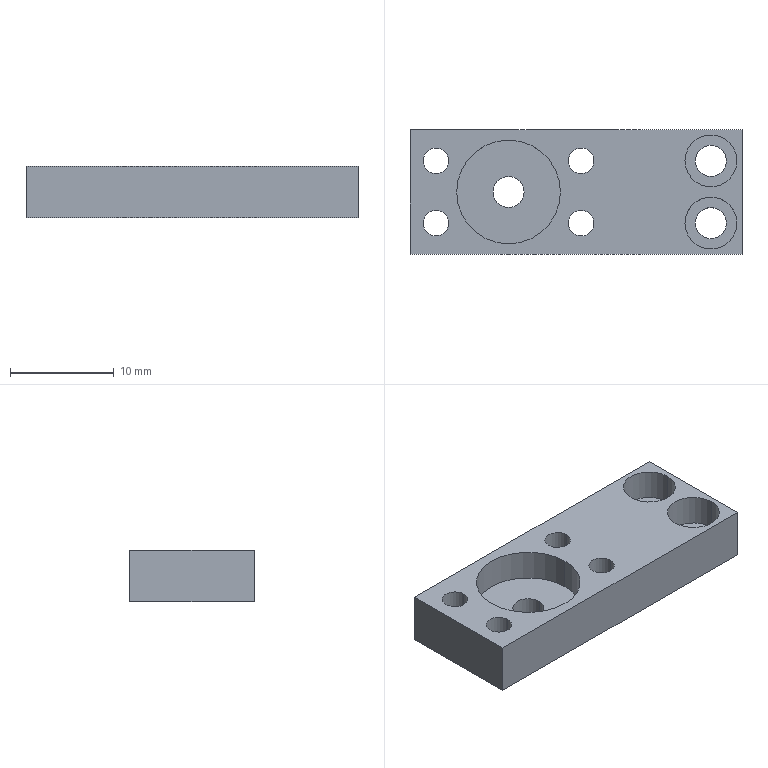Part | SolidWorks | features BaseBody 1 | 1 solid | 29 faces | box 32 x 12 x 5 mm | volume 1429 mm3 | cylinder 20 | plane 9 | commonest cylinder face diameters 2.459 x8 3 x6 5 x4 10 x2
STEP:
#1=CARTESIAN_POINT('',(12.928,0.6763,0.));
#2=VERTEX_POINT('',#1);
#3=CARTESIAN_POINT('',(9.928,0.6763,0.));
#4=VERTEX_POINT('',#3);
#5=CARTESIAN_POINT('',(11.428,0.6763,0.));
#6=DIRECTION('',(0.,0.,-1.));
#7=DIRECTION('',(1.,0.,0.));
#8=AXIS2_PLACEMENT_3D('',#5,#6,#7);
#9=CIRCLE('',#8,1.5);
#10=EDGE_CURVE('',#2,#4,#9,.T.);
#11=ORIENTED_EDGE('',*,*,#10,.T.);
#12=CARTESIAN_POINT('',(9.928,0.6763,2.));
#13=VERTEX_POINT('',#12);
#14=CARTESIAN_POINT('',(9.928,0.6763,-29.54));
#15=DIRECTION('',(0.,0.,1.));
#16=VECTOR('',#15,1000.);
#17=LINE('',#14,#16);
#18=EDGE_CURVE('',#4,#13,#17,.T.);
#19=ORIENTED_EDGE('',*,*,#18,.T.);
#20=CARTESIAN_POINT('',(12.928,0.6763,2.));
#21=VERTEX_POINT('',#20);
#22=CARTESIAN_POINT('',(11.428,0.6763,2.));
#23=DIRECTION('',(0.,0.,-1.));
#24=DIRECTION('',(1.,0.,0.));
#25=AXIS2_PLACEMENT_3D('',#22,#23,#24);
#26=CIRCLE('',#25,1.5);
#27=EDGE_CURVE('',#21,#13,#26,.T.);
#28=ORIENTED_EDGE('',*,*,#27,.F.);
#29=CARTESIAN_POINT('',(12.928,0.6763,-29.54));
#30=DIRECTION('',(0.,0.,1.));
#31=VECTOR('',#30,1000.);
#32=LINE('',#29,#31);
#33=EDGE_CURVE('',#2,#21,#32,.T.);
#34=ORIENTED_EDGE('',*,*,#33,.F.);
#35=EDGE_LOOP('',(#11,#19,#28,#34));
#36=FACE_OUTER_BOUND('',#35,.T.);
#37=CARTESIAN_POINT('',(11.428,0.6763,-29.54));
#38=DIRECTION('',(0.,0.,1.));
#39=DIRECTION('',(1.,0.,0.));
#40=AXIS2_PLACEMENT_3D('',#37,#38,#39);
#41=CYLINDRICAL_SURFACE('',#40,1.5);
#42=ADVANCED_FACE('',(#36),#41,.F.);
#43=CARTESIAN_POINT('',(12.928,-5.324,0.));
#44=VERTEX_POINT('',#43);
#45=CARTESIAN_POINT('',(9.928,-5.324,0.));
#46=VERTEX_POINT('',#45);
#47=CARTESIAN_POINT('',(11.428,-5.324,0.));
#48=DIRECTION('',(0.,0.,-1.));
#49=DIRECTION('',(1.,0.,0.));
#50=AXIS2_PLACEMENT_3D('',#47,#48,#49);
#51=CIRCLE('',#50,1.5);
#52=EDGE_CURVE('',#44,#46,#51,.T.);
#53=ORIENTED_EDGE('',*,*,#52,.T.);
#54=CARTESIAN_POINT('',(9.928,-5.324,2.));
#55=VERTEX_POINT('',#54);
#56=CARTESIAN_POINT('',(9.928,-5.324,-29.54));
#57=DIRECTION('',(0.,0.,1.));
#58=VECTOR('',#57,1000.);
#59=LINE('',#56,#58);
#60=EDGE_CURVE('',#46,#55,#59,.T.);
#61=ORIENTED_EDGE('',*,*,#60,.T.);
#62=CARTESIAN_POINT('',(12.928,-5.324,2.));
#63=VERTEX_POINT('',#62);
#64=CARTESIAN_POINT('',(11.428,-5.324,2.));
#65=DIRECTION('',(0.,0.,-1.));
#66=DIRECTION('',(1.,0.,0.));
#67=AXIS2_PLACEMENT_3D('',#64,#65,#66);
#68=CIRCLE('',#67,1.5);
#69=EDGE_CURVE('',#63,#55,#68,.T.);
#70=ORIENTED_EDGE('',*,*,#69,.F.);
#71=CARTESIAN_POINT('',(12.928,-5.324,-29.54));
#72=DIRECTION('',(0.,0.,1.));
#73=VECTOR('',#72,1000.);
#74=LINE('',#71,#73);
#75=EDGE_CURVE('',#44,#63,#74,.T.);
#76=ORIENTED_EDGE('',*,*,#75,.F.);
#77=EDGE_LOOP('',(#53,#61,#70,#76));
#78=FACE_OUTER_BOUND('',#77,.T.);
#79=CARTESIAN_POINT('',(11.428,-5.324,-29.54));
#80=DIRECTION('',(0.,0.,1.));
#81=DIRECTION('',(1.,0.,0.));
#82=AXIS2_PLACEMENT_3D('',#79,#80,#81);
#83=CYLINDRICAL_SURFACE('',#82,1.5);
#84=ADVANCED_FACE('',(#78),#83,.F.);
#85=CARTESIAN_POINT('',(-6.572,-2.324,0.));
#86=VERTEX_POINT('',#85);
#87=CARTESIAN_POINT('',(-9.572,-2.324,0.));
#88=VERTEX_POINT('',#87);
#89=CARTESIAN_POINT('',(-8.072,-2.324,0.));
#90=DIRECTION('',(0.,0.,-1.));
#91=DIRECTION('',(1.,0.,0.));
#92=AXIS2_PLACEMENT_3D('',#89,#90,#91);
#93=CIRCLE('',#92,1.5);
#94=EDGE_CURVE('',#86,#88,#93,.T.);
#95=ORIENTED_EDGE('',*,*,#94,.T.);
#96=CARTESIAN_POINT('',(-9.572,-2.324,2.));
#97=VERTEX_POINT('',#96);
#98=CARTESIAN_POINT('',(-9.572,-2.324,-29.54));
#99=DIRECTION('',(0.,0.,1.));
#100=VECTOR('',#99,1000.);
#101=LINE('',#98,#100);
#102=EDGE_CURVE('',#88,#97,#101,.T.);
#103=ORIENTED_EDGE('',*,*,#102,.T.);
#104=CARTESIAN_POINT('',(-6.572,-2.324,2.));
#105=VERTEX_POINT('',#104);
#106=CARTESIAN_POINT('',(-8.072,-2.324,2.));
#107=DIRECTION('',(0.,0.,-1.));
#108=DIRECTION('',(1.,0.,0.));
#109=AXIS2_PLACEMENT_3D('',#106,#107,#108);
#110=CIRCLE('',#109,1.5);
#111=EDGE_CURVE('',#105,#97,#110,.T.);
#112=ORIENTED_EDGE('',*,*,#111,.F.);
#113=CARTESIAN_POINT('',(-6.572,-2.324,-29.54));
#114=DIRECTION('',(0.,0.,1.));
#115=VECTOR('',#114,1000.);
#116=LINE('',#113,#115);
#117=EDGE_CURVE('',#86,#105,#116,.T.);
#118=ORIENTED_EDGE('',*,*,#117,.F.);
#119=EDGE_LOOP('',(#95,#103,#112,#118));
#120=FACE_OUTER_BOUND('',#119,.T.);
#121=CARTESIAN_POINT('',(-8.072,-2.324,-29.54));
#122=DIRECTION('',(0.,0.,1.));
#123=DIRECTION('',(1.,0.,0.));
#124=AXIS2_PLACEMENT_3D('',#121,#122,#123);
#125=CYLINDRICAL_SURFACE('',#124,1.5);
#126=ADVANCED_FACE('',(#120),#125,.F.);
#127=CARTESIAN_POINT('',(-13.843,0.6763,0.));
#128=VERTEX_POINT('',#127);
#129=CARTESIAN_POINT('',(-16.302,0.6763,0.));
#130=VERTEX_POINT('',#129);
#131=CARTESIAN_POINT('',(-15.072,0.6763,0.));
#132=DIRECTION('',(0.,0.,-1.));
#133=DIRECTION('',(1.,0.,0.));
#134=AXIS2_PLACEMENT_3D('',#131,#132,#133);
#135=CIRCLE('',#134,1.229);
#136=EDGE_CURVE('',#128,#130,#135,.T.);
#137=ORIENTED_EDGE('',*,*,#136,.T.);
#138=CARTESIAN_POINT('',(-16.302,0.6763,5.));
#139=VERTEX_POINT('',#138);
#140=CARTESIAN_POINT('',(-16.302,0.6763,-29.54));
#141=DIRECTION('',(0.,0.,1.));
#142=VECTOR('',#141,1000.);
#143=LINE('',#140,#142);
#144=EDGE_CURVE('',#130,#139,#143,.T.);
#145=ORIENTED_EDGE('',*,*,#144,.T.);
#146=CARTESIAN_POINT('',(-13.843,0.6763,5.));
#147=VERTEX_POINT('',#146);
#148=CARTESIAN_POINT('',(-15.072,0.6763,5.));
#149=DIRECTION('',(0.,0.,-1.));
#150=DIRECTION('',(1.,0.,0.));
#151=AXIS2_PLACEMENT_3D('',#148,#149,#150);
#152=CIRCLE('',#151,1.229);
#153=EDGE_CURVE('',#147,#139,#152,.T.);
#154=ORIENTED_EDGE('',*,*,#153,.F.);
#155=CARTESIAN_POINT('',(-13.843,0.6763,-29.54));
#156=DIRECTION('',(0.,0.,1.));
#157=VECTOR('',#156,1000.);
#158=LINE('',#155,#157);
#159=EDGE_CURVE('',#128,#147,#158,.T.);
#160=ORIENTED_EDGE('',*,*,#159,.F.);
#161=EDGE_LOOP('',(#137,#145,#154,#160));
#162=FACE_OUTER_BOUND('',#161,.T.);
#163=CARTESIAN_POINT('',(-15.072,0.6763,-29.54));
#164=DIRECTION('',(0.,0.,1.));
#165=DIRECTION('',(1.,0.,0.));
#166=AXIS2_PLACEMENT_3D('',#163,#164,#165);
#167=CYLINDRICAL_SURFACE('',#166,1.229);
#168=ADVANCED_FACE('',(#162),#167,.F.);
#169=CARTESIAN_POINT('',(0.1572,0.6763,0.));
#170=VERTEX_POINT('',#169);
#171=CARTESIAN_POINT('',(-2.302,0.6763,0.));
#172=VERTEX_POINT('',#171);
#173=CARTESIAN_POINT('',(-1.072,0.6763,0.));
#174=DIRECTION('',(0.,0.,-1.));
#175=DIRECTION('',(1.,0.,0.));
#176=AXIS2_PLACEMENT_3D('',#173,#174,#175);
#177=CIRCLE('',#176,1.23);
#178=EDGE_CURVE('',#170,#172,#177,.T.);
#179=ORIENTED_EDGE('',*,*,#178,.T.);
#180=CARTESIAN_POINT('',(-2.302,0.6763,5.));
#181=VERTEX_POINT('',#180);
#182=CARTESIAN_POINT('',(-2.302,0.6763,-29.54));
#183=DIRECTION('',(0.,0.,1.));
#184=VECTOR('',#183,1000.);
#185=LINE('',#182,#184);
#186=EDGE_CURVE('',#172,#181,#185,.T.);
#187=ORIENTED_EDGE('',*,*,#186,.T.);
#188=CARTESIAN_POINT('',(0.1572,0.6763,5.));
#189=VERTEX_POINT('',#188);
#190=CARTESIAN_POINT('',(-1.072,0.6763,5.));
#191=DIRECTION('',(0.,0.,-1.));
#192=DIRECTION('',(1.,0.,0.));
#193=AXIS2_PLACEMENT_3D('',#190,#191,#192);
#194=CIRCLE('',#193,1.23);
#195=EDGE_CURVE('',#189,#181,#194,.T.);
#196=ORIENTED_EDGE('',*,*,#195,.F.);
#197=CARTESIAN_POINT('',(0.1572,0.6763,-29.54));
#198=DIRECTION('',(0.,0.,1.));
#199=VECTOR('',#198,1000.);
#200=LINE('',#197,#199);
#201=EDGE_CURVE('',#170,#189,#200,.T.);
#202=ORIENTED_EDGE('',*,*,#201,.F.);
#203=EDGE_LOOP('',(#179,#187,#196,#202));
#204=FACE_OUTER_BOUND('',#203,.T.);
#205=CARTESIAN_POINT('',(-1.072,0.6763,-29.54));
#206=DIRECTION('',(0.,0.,1.));
#207=DIRECTION('',(1.,0.,0.));
#208=AXIS2_PLACEMENT_3D('',#205,#206,#207);
#209=CYLINDRICAL_SURFACE('',#208,1.23);
#210=ADVANCED_FACE('',(#204),#209,.F.);
#211=CARTESIAN_POINT('',(0.1572,-5.324,0.));
#212=VERTEX_POINT('',#211);
#213=CARTESIAN_POINT('',(-2.302,-5.324,0.));
#214=VERTEX_POINT('',#213);
#215=CARTESIAN_POINT('',(-1.072,-5.324,0.));
#216=DIRECTION('',(0.,0.,-1.));
#217=DIRECTION('',(1.,0.,0.));
#218=AXIS2_PLACEMENT_3D('',#215,#216,#217);
#219=CIRCLE('',#218,1.23);
#220=EDGE_CURVE('',#212,#214,#219,.T.);
#221=ORIENTED_EDGE('',*,*,#220,.T.);
#222=CARTESIAN_POINT('',(-2.302,-5.324,5.));
#223=VERTEX_POINT('',#222);
#224=CARTESIAN_POINT('',(-2.302,-5.324,-29.54));
#225=DIRECTION('',(0.,0.,1.));
#226=VECTOR('',#225,1000.);
#227=LINE('',#224,#226);
#228=EDGE_CURVE('',#214,#223,#227,.T.);
#229=ORIENTED_EDGE('',*,*,#228,.T.);
#230=CARTESIAN_POINT('',(0.1572,-5.324,5.));
#231=VERTEX_POINT('',#230);
#232=CARTESIAN_POINT('',(-1.072,-5.324,5.));
#233=DIRECTION('',(0.,0.,-1.));
#234=DIRECTION('',(1.,0.,0.));
#235=AXIS2_PLACEMENT_3D('',#232,#233,#234);
#236=CIRCLE('',#235,1.23);
#237=EDGE_CURVE('',#231,#223,#236,.T.);
#238=ORIENTED_EDGE('',*,*,#237,.F.);
#239=CARTESIAN_POINT('',(0.1572,-5.324,-29.54));
#240=DIRECTION('',(0.,0.,1.));
#241=VECTOR('',#240,1000.);
#242=LINE('',#239,#241);
#243=EDGE_CURVE('',#212,#231,#242,.T.);
#244=ORIENTED_EDGE('',*,*,#243,.F.);
#245=EDGE_LOOP('',(#221,#229,#238,#244));
#246=FACE_OUTER_BOUND('',#245,.T.);
#247=CARTESIAN_POINT('',(-1.072,-5.324,-29.54));
#248=DIRECTION('',(0.,0.,1.));
#249=DIRECTION('',(1.,0.,0.));
#250=AXIS2_PLACEMENT_3D('',#247,#248,#249);
#251=CYLINDRICAL_SURFACE('',#250,1.23);
#252=ADVANCED_FACE('',(#246),#251,.F.);
#253=CARTESIAN_POINT('',(-13.843,-5.324,0.));
#254=VERTEX_POINT('',#253);
#255=CARTESIAN_POINT('',(-16.302,-5.324,0.));
#256=VERTEX_POINT('',#255);
#257=CARTESIAN_POINT('',(-15.072,-5.324,0.));
#258=DIRECTION('',(0.,0.,-1.));
#259=DIRECTION('',(1.,0.,0.));
#260=AXIS2_PLACEMENT_3D('',#257,#258,#259);
#261=CIRCLE('',#260,1.229);
#262=EDGE_CURVE('',#254,#256,#261,.T.);
#263=ORIENTED_EDGE('',*,*,#262,.T.);
#264=CARTESIAN_POINT('',(-16.302,-5.324,5.));
#265=VERTEX_POINT('',#264);
#266=CARTESIAN_POINT('',(-16.302,-5.324,-29.54));
#267=DIRECTION('',(0.,0.,1.));
#268=VECTOR('',#267,1000.);
#269=LINE('',#266,#268);
#270=EDGE_CURVE('',#256,#265,#269,.T.);
#271=ORIENTED_EDGE('',*,*,#270,.T.);
#272=CARTESIAN_POINT('',(-13.843,-5.324,5.));
#273=VERTEX_POINT('',#272);
#274=CARTESIAN_POINT('',(-15.072,-5.324,5.));
#275=DIRECTION('',(0.,0.,-1.));
#276=DIRECTION('',(1.,0.,0.));
#277=AXIS2_PLACEMENT_3D('',#274,#275,#276);
#278=CIRCLE('',#277,1.229);
#279=EDGE_CURVE('',#273,#265,#278,.T.);
#280=ORIENTED_EDGE('',*,*,#279,.F.);
#281=CARTESIAN_POINT('',(-13.843,-5.324,-29.54));
#282=DIRECTION('',(0.,0.,1.));
#283=VECTOR('',#282,1000.);
#284=LINE('',#281,#283);
#285=EDGE_CURVE('',#254,#273,#284,.T.);
#286=ORIENTED_EDGE('',*,*,#285,.F.);
#287=EDGE_LOOP('',(#263,#271,#280,#286));
#288=FACE_OUTER_BOUND('',#287,.T.);
#289=CARTESIAN_POINT('',(-15.072,-5.324,-29.54));
#290=DIRECTION('',(0.,0.,1.));
#291=DIRECTION('',(1.,0.,0.));
#292=AXIS2_PLACEMENT_3D('',#289,#290,#291);
#293=CYLINDRICAL_SURFACE('',#292,1.229);
#294=ADVANCED_FACE('',(#288),#293,.F.);
#295=CARTESIAN_POINT('',(8.928,0.6763,2.));
#296=VERTEX_POINT('',#295);
#297=CARTESIAN_POINT('',(13.928,0.6763,2.));
#298=VERTEX_POINT('',#297);
#299=CARTESIAN_POINT('',(11.428,0.6763,2.));
#300=DIRECTION('',(0.,0.,1.));
#301=DIRECTION('',(1.,0.,0.));
#302=AXIS2_PLACEMENT_3D('',#299,#300,#301);
#303=CIRCLE('',#302,2.5);
#304=EDGE_CURVE('',#296,#298,#303,.T.);
#305=ORIENTED_EDGE('',*,*,#304,.F.);
#306=CARTESIAN_POINT('',(8.928,0.6763,5.));
#307=VERTEX_POINT('',#306);
#308=CARTESIAN_POINT('',(8.928,0.6763,3.5));
#309=DIRECTION('',(0.,0.,1.));
#310=VECTOR('',#309,1000.);
#311=LINE('',#308,#310);
#312=EDGE_CURVE('',#296,#307,#311,.T.);
#313=ORIENTED_EDGE('',*,*,#312,.T.);
#314=CARTESIAN_POINT('',(13.928,0.6763,5.));
#315=VERTEX_POINT('',#314);
#316=CARTESIAN_POINT('',(11.428,0.6763,5.));
#317=DIRECTION('',(0.,0.,-1.));
#318=DIRECTION('',(1.,0.,0.));
#319=AXIS2_PLACEMENT_3D('',#316,#317,#318);
#320=CIRCLE('',#319,2.5);
#321=EDGE_CURVE('',#315,#307,#320,.T.);
#322=ORIENTED_EDGE('',*,*,#321,.F.);
#323=CARTESIAN_POINT('',(13.928,0.6763,3.5));
#324=DIRECTION('',(0.,0.,1.));
#325=VECTOR('',#324,1000.);
#326=LINE('',#323,#325);
#327=EDGE_CURVE('',#298,#315,#326,.T.);
#328=ORIENTED_EDGE('',*,*,#327,.F.);
#329=EDGE_LOOP('',(#305,#313,#322,#328));
#330=FACE_OUTER_BOUND('',#329,.T.);
#331=CARTESIAN_POINT('',(11.428,0.6763,3.5));
#332=DIRECTION('',(0.,0.,1.));
#333=DIRECTION('',(1.,0.,0.));
#334=AXIS2_PLACEMENT_3D('',#331,#332,#333);
#335=CYLINDRICAL_SURFACE('',#334,2.5);
#336=ADVANCED_FACE('',(#330),#335,.F.);
#337=CARTESIAN_POINT('',(8.928,-5.324,2.));
#338=VERTEX_POINT('',#337);
#339=CARTESIAN_POINT('',(13.928,-5.324,2.));
#340=VERTEX_POINT('',#339);
#341=CARTESIAN_POINT('',(11.428,-5.324,2.));
#342=DIRECTION('',(0.,0.,1.));
#343=DIRECTION('',(1.,0.,0.));
#344=AXIS2_PLACEMENT_3D('',#341,#342,#343);
#345=CIRCLE('',#344,2.5);
#346=EDGE_CURVE('',#338,#340,#345,.T.);
#347=ORIENTED_EDGE('',*,*,#346,.F.);
#348=CARTESIAN_POINT('',(8.928,-5.324,5.));
#349=VERTEX_POINT('',#348);
#350=CARTESIAN_POINT('',(8.928,-5.324,3.5));
#351=DIRECTION('',(0.,0.,1.));
#352=VECTOR('',#351,1000.);
#353=LINE('',#350,#352);
#354=EDGE_CURVE('',#338,#349,#353,.T.);
#355=ORIENTED_EDGE('',*,*,#354,.T.);
#356=CARTESIAN_POINT('',(13.928,-5.324,5.));
#357=VERTEX_POINT('',#356);
#358=CARTESIAN_POINT('',(11.428,-5.324,5.));
#359=DIRECTION('',(0.,0.,-1.));
#360=DIRECTION('',(1.,0.,0.));
#361=AXIS2_PLACEMENT_3D('',#358,#359,#360);
#362=CIRCLE('',#361,2.5);
#363=EDGE_CURVE('',#357,#349,#362,.T.);
#364=ORIENTED_EDGE('',*,*,#363,.F.);
#365=CARTESIAN_POINT('',(13.928,-5.324,3.5));
#366=DIRECTION('',(0.,0.,1.));
#367=VECTOR('',#366,1000.);
#368=LINE('',#365,#367);
#369=EDGE_CURVE('',#340,#357,#368,.T.);
#370=ORIENTED_EDGE('',*,*,#369,.F.);
#371=EDGE_LOOP('',(#347,#355,#364,#370));
#372=FACE_OUTER_BOUND('',#371,.T.);
#373=CARTESIAN_POINT('',(11.428,-5.324,3.5));
#374=DIRECTION('',(0.,0.,1.));
#375=DIRECTION('',(1.,0.,0.));
#376=AXIS2_PLACEMENT_3D('',#373,#374,#375);
#377=CYLINDRICAL_SURFACE('',#376,2.5);
#378=ADVANCED_FACE('',(#372),#377,.F.);
#379=CARTESIAN_POINT('',(-13.072,-2.324,2.));
#380=VERTEX_POINT('',#379);
#381=CARTESIAN_POINT('',(-3.072,-2.324,2.));
#382=VERTEX_POINT('',#381);
#383=CARTESIAN_POINT('',(-8.072,-2.324,2.));
#384=DIRECTION('',(0.,0.,1.));
#385=DIRECTION('',(1.,0.,0.));
#386=AXIS2_PLACEMENT_3D('',#383,#384,#385);
#387=CIRCLE('',#386,5.);
#388=EDGE_CURVE('',#380,#382,#387,.T.);
#389=ORIENTED_EDGE('',*,*,#388,.F.);
#390=CARTESIAN_POINT('',(-13.072,-2.324,5.));
#391=VERTEX_POINT('',#390);
#392=CARTESIAN_POINT('',(-13.072,-2.324,3.5));
#393=DIRECTION('',(0.,0.,1.));
#394=VECTOR('',#393,1000.);
#395=LINE('',#392,#394);
#396=EDGE_CURVE('',#380,#391,#395,.T.);
#397=ORIENTED_EDGE('',*,*,#396,.T.);
#398=CARTESIAN_POINT('',(-3.072,-2.324,5.));
#399=VERTEX_POINT('',#398);
#400=CARTESIAN_POINT('',(-8.072,-2.324,5.));
#401=DIRECTION('',(0.,0.,-1.));
#402=DIRECTION('',(1.,0.,0.));
#403=AXIS2_PLACEMENT_3D('',#400,#401,#402);
#404=CIRCLE('',#403,5.);
#405=EDGE_CURVE('',#399,#391,#404,.T.);
#406=ORIENTED_EDGE('',*,*,#405,.F.);
#407=CARTESIAN_POINT('',(-3.072,-2.324,3.5));
#408=DIRECTION('',(0.,0.,1.));
#409=VECTOR('',#408,1000.);
#410=LINE('',#407,#409);
#411=EDGE_CURVE('',#382,#399,#410,.T.);
#412=ORIENTED_EDGE('',*,*,#411,.F.);
#413=EDGE_LOOP('',(#389,#397,#406,#412));
#414=FACE_OUTER_BOUND('',#413,.T.);
#415=CARTESIAN_POINT('',(-8.072,-2.324,3.5));
#416=DIRECTION('',(0.,0.,1.));
#417=DIRECTION('',(1.,0.,0.));
#418=AXIS2_PLACEMENT_3D('',#415,#416,#417);
#419=CYLINDRICAL_SURFACE('',#418,5.);
#420=ADVANCED_FACE('',(#414),#419,.F.);
#421=ORIENTED_EDGE('',*,*,#10,.F.);
#422=CARTESIAN_POINT('',(11.428,0.6763,0.));
#423=DIRECTION('',(0.,0.,-1.));
#424=DIRECTION('',(1.,0.,0.));
#425=AXIS2_PLACEMENT_3D('',#422,#423,#424);
#426=CIRCLE('',#425,1.5);
#427=EDGE_CURVE('',#4,#2,#426,.T.);
#428=ORIENTED_EDGE('',*,*,#427,.F.);
#429=EDGE_LOOP('',(#421,#428));
#430=FACE_BOUND('',#429,.T.);
#431=ORIENTED_EDGE('',*,*,#52,.F.);
#432=CARTESIAN_POINT('',(11.428,-5.324,0.));
#433=DIRECTION('',(0.,0.,-1.));
#434=DIRECTION('',(1.,0.,0.));
#435=AXIS2_PLACEMENT_3D('',#432,#433,#434);
#436=CIRCLE('',#435,1.5);
#437=EDGE_CURVE('',#46,#44,#436,.T.);
#438=ORIENTED_EDGE('',*,*,#437,.F.);
#439=EDGE_LOOP('',(#431,#438));
#440=FACE_BOUND('',#439,.T.);
#441=ORIENTED_EDGE('',*,*,#94,.F.);
#442=CARTESIAN_POINT('',(-8.072,-2.324,0.));
#443=DIRECTION('',(0.,0.,-1.));
#444=DIRECTION('',(1.,0.,0.));
#445=AXIS2_PLACEMENT_3D('',#442,#443,#444);
#446=CIRCLE('',#445,1.5);
#447=EDGE_CURVE('',#88,#86,#446,.T.);
#448=ORIENTED_EDGE('',*,*,#447,.F.);
#449=EDGE_LOOP('',(#441,#448));
#450=FACE_BOUND('',#449,.T.);
#451=ORIENTED_EDGE('',*,*,#136,.F.);
#452=CARTESIAN_POINT('',(-15.072,0.6763,0.));
#453=DIRECTION('',(0.,0.,-1.));
#454=DIRECTION('',(1.,0.,0.));
#455=AXIS2_PLACEMENT_3D('',#452,#453,#454);
#456=CIRCLE('',#455,1.229);
#457=EDGE_CURVE('',#130,#128,#456,.T.);
#458=ORIENTED_EDGE('',*,*,#457,.F.);
#459=EDGE_LOOP('',(#451,#458));
#460=FACE_BOUND('',#459,.T.);
#461=ORIENTED_EDGE('',*,*,#178,.F.);
#462=CARTESIAN_POINT('',(-1.072,0.6763,0.));
#463=DIRECTION('',(0.,0.,-1.));
#464=DIRECTION('',(1.,0.,0.));
#465=AXIS2_PLACEMENT_3D('',#462,#463,#464);
#466=CIRCLE('',#465,1.23);
#467=EDGE_CURVE('',#172,#170,#466,.T.);
#468=ORIENTED_EDGE('',*,*,#467,.F.);
#469=EDGE_LOOP('',(#461,#468));
#470=FACE_BOUND('',#469,.T.);
#471=ORIENTED_EDGE('',*,*,#220,.F.);
#472=CARTESIAN_POINT('',(-1.072,-5.324,0.));
#473=DIRECTION('',(0.,0.,-1.));
#474=DIRECTION('',(1.,0.,0.));
#475=AXIS2_PLACEMENT_3D('',#472,#473,#474);
#476=CIRCLE('',#475,1.23);
#477=EDGE_CURVE('',#214,#212,#476,.T.);
#478=ORIENTED_EDGE('',*,*,#477,.F.);
#479=EDGE_LOOP('',(#471,#478));
#480=FACE_BOUND('',#479,.T.);
#481=ORIENTED_EDGE('',*,*,#262,.F.);
#482=CARTESIAN_POINT('',(-15.072,-5.324,0.));
#483=DIRECTION('',(0.,0.,-1.));
#484=DIRECTION('',(1.,0.,0.));
#485=AXIS2_PLACEMENT_3D('',#482,#483,#484);
#486=CIRCLE('',#485,1.229);
#487=EDGE_CURVE('',#256,#254,#486,.T.);
#488=ORIENTED_EDGE('',*,*,#487,.F.);
#489=EDGE_LOOP('',(#481,#488));
#490=FACE_BOUND('',#489,.T.);
#491=CARTESIAN_POINT('',(14.428,-8.324,0.));
#492=VERTEX_POINT('',#491);
#493=CARTESIAN_POINT('',(14.428,3.676,0.));
#494=VERTEX_POINT('',#493);
#495=CARTESIAN_POINT('',(14.428,-2.324,0.));
#496=DIRECTION('',(0.,1.,0.));
#497=VECTOR('',#496,1000.);
#498=LINE('',#495,#497);
#499=EDGE_CURVE('',#492,#494,#498,.T.);
#500=ORIENTED_EDGE('',*,*,#499,.F.);
#501=CARTESIAN_POINT('',(-17.572,-8.324,0.));
#502=VERTEX_POINT('',#501);
#503=CARTESIAN_POINT('',(-1.572,-8.324,0.));
#504=DIRECTION('',(1.,0.,0.));
#505=VECTOR('',#504,1000.);
#506=LINE('',#503,#505);
#507=EDGE_CURVE('',#502,#492,#506,.T.);
#508=ORIENTED_EDGE('',*,*,#507,.F.);
#509=CARTESIAN_POINT('',(-17.572,3.676,0.));
#510=VERTEX_POINT('',#509);
#511=CARTESIAN_POINT('',(-17.572,-2.324,0.));
#512=DIRECTION('',(0.,-1.,0.));
#513=VECTOR('',#512,1000.);
#514=LINE('',#511,#513);
#515=EDGE_CURVE('',#510,#502,#514,.T.);
#516=ORIENTED_EDGE('',*,*,#515,.F.);
#517=CARTESIAN_POINT('',(-1.572,3.676,0.));
#518=DIRECTION('',(-1.,0.,0.));
#519=VECTOR('',#518,1000.);
#520=LINE('',#517,#519);
#521=EDGE_CURVE('',#494,#510,#520,.T.);
#522=ORIENTED_EDGE('',*,*,#521,.F.);
#523=EDGE_LOOP('',(#500,#508,#516,#522));
#524=FACE_OUTER_BOUND('',#523,.T.);
#525=CARTESIAN_POINT('',(-1.572,-2.324,0.));
#526=DIRECTION('',(0.,0.,1.));
#527=DIRECTION('',(1.,0.,0.));
#528=AXIS2_PLACEMENT_3D('',#525,#526,#527);
#529=PLANE('',#528);
#530=ADVANCED_FACE('',(#430,#440,#450,#460,#470,#480,#490,#524),#529,.F.);
#531=ORIENTED_EDGE('',*,*,#18,.F.);
#532=ORIENTED_EDGE('',*,*,#427,.T.);
#533=ORIENTED_EDGE('',*,*,#33,.T.);
#534=CARTESIAN_POINT('',(11.428,0.6763,2.));
#535=DIRECTION('',(0.,0.,-1.));
#536=DIRECTION('',(1.,0.,0.));
#537=AXIS2_PLACEMENT_3D('',#534,#535,#536);
#538=CIRCLE('',#537,1.5);
#539=EDGE_CURVE('',#13,#21,#538,.T.);
#540=ORIENTED_EDGE('',*,*,#539,.F.);
#541=EDGE_LOOP('',(#531,#532,#533,#540));
#542=FACE_OUTER_BOUND('',#541,.T.);
#543=CARTESIAN_POINT('',(11.428,0.6763,-29.54));
#544=DIRECTION('',(0.,0.,1.));
#545=DIRECTION('',(1.,0.,0.));
#546=AXIS2_PLACEMENT_3D('',#543,#544,#545);
#547=CYLINDRICAL_SURFACE('',#546,1.5);
#548=ADVANCED_FACE('',(#542),#547,.F.);
#549=ORIENTED_EDGE('',*,*,#60,.F.);
#550=ORIENTED_EDGE('',*,*,#437,.T.);
#551=ORIENTED_EDGE('',*,*,#75,.T.);
#552=CARTESIAN_POINT('',(11.428,-5.324,2.));
#553=DIRECTION('',(0.,0.,-1.));
#554=DIRECTION('',(1.,0.,0.));
#555=AXIS2_PLACEMENT_3D('',#552,#553,#554);
#556=CIRCLE('',#555,1.5);
#557=EDGE_CURVE('',#55,#63,#556,.T.);
#558=ORIENTED_EDGE('',*,*,#557,.F.);
#559=EDGE_LOOP('',(#549,#550,#551,#558));
#560=FACE_OUTER_BOUND('',#559,.T.);
#561=CARTESIAN_POINT('',(11.428,-5.324,-29.54));
#562=DIRECTION('',(0.,0.,1.));
#563=DIRECTION('',(1.,0.,0.));
#564=AXIS2_PLACEMENT_3D('',#561,#562,#563);
#565=CYLINDRICAL_SURFACE('',#564,1.5);
#566=ADVANCED_FACE('',(#560),#565,.F.);
#567=ORIENTED_EDGE('',*,*,#102,.F.);
#568=ORIENTED_EDGE('',*,*,#447,.T.);
#569=ORIENTED_EDGE('',*,*,#117,.T.);
#570=CARTESIAN_POINT('',(-8.072,-2.324,2.));
#571=DIRECTION('',(0.,0.,-1.));
#572=DIRECTION('',(1.,0.,0.));
#573=AXIS2_PLACEMENT_3D('',#570,#571,#572);
#574=CIRCLE('',#573,1.5);
#575=EDGE_CURVE('',#97,#105,#574,.T.);
#576=ORIENTED_EDGE('',*,*,#575,.F.);
#577=EDGE_LOOP('',(#567,#568,#569,#576));
#578=FACE_OUTER_BOUND('',#577,.T.);
#579=CARTESIAN_POINT('',(-8.072,-2.324,-29.54));
#580=DIRECTION('',(0.,0.,1.));
#581=DIRECTION('',(1.,0.,0.));
#582=AXIS2_PLACEMENT_3D('',#579,#580,#581);
#583=CYLINDRICAL_SURFACE('',#582,1.5);
#584=ADVANCED_FACE('',(#578),#583,.F.);
#585=ORIENTED_EDGE('',*,*,#144,.F.);
#586=ORIENTED_EDGE('',*,*,#457,.T.);
#587=ORIENTED_EDGE('',*,*,#159,.T.);
#588=CARTESIAN_POINT('',(-15.072,0.6763,5.));
#589=DIRECTION('',(0.,0.,-1.));
#590=DIRECTION('',(1.,0.,0.));
#591=AXIS2_PLACEMENT_3D('',#588,#589,#590);
#592=CIRCLE('',#591,1.229);
#593=EDGE_CURVE('',#139,#147,#592,.T.);
#594=ORIENTED_EDGE('',*,*,#593,.F.);
#595=EDGE_LOOP('',(#585,#586,#587,#594));
#596=FACE_OUTER_BOUND('',#595,.T.);
#597=CARTESIAN_POINT('',(-15.072,0.6763,-29.54));
#598=DIRECTION('',(0.,0.,1.));
#599=DIRECTION('',(1.,0.,0.));
#600=AXIS2_PLACEMENT_3D('',#597,#598,#599);
#601=CYLINDRICAL_SURFACE('',#600,1.229);
#602=ADVANCED_FACE('',(#596),#601,.F.);
#603=ORIENTED_EDGE('',*,*,#186,.F.);
#604=ORIENTED_EDGE('',*,*,#467,.T.);
#605=ORIENTED_EDGE('',*,*,#201,.T.);
#606=CARTESIAN_POINT('',(-1.072,0.6763,5.));
#607=DIRECTION('',(0.,0.,-1.));
#608=DIRECTION('',(1.,0.,0.));
#609=AXIS2_PLACEMENT_3D('',#606,#607,#608);
#610=CIRCLE('',#609,1.23);
#611=EDGE_CURVE('',#181,#189,#610,.T.);
#612=ORIENTED_EDGE('',*,*,#611,.F.);
#613=EDGE_LOOP('',(#603,#604,#605,#612));
#614=FACE_OUTER_BOUND('',#613,.T.);
#615=CARTESIAN_POINT('',(-1.072,0.6763,-29.54));
#616=DIRECTION('',(0.,0.,1.));
#617=DIRECTION('',(1.,0.,0.));
#618=AXIS2_PLACEMENT_3D('',#615,#616,#617);
#619=CYLINDRICAL_SURFACE('',#618,1.23);
#620=ADVANCED_FACE('',(#614),#619,.F.);
#621=ORIENTED_EDGE('',*,*,#228,.F.);
#622=ORIENTED_EDGE('',*,*,#477,.T.);
#623=ORIENTED_EDGE('',*,*,#243,.T.);
#624=CARTESIAN_POINT('',(-1.072,-5.324,5.));
#625=DIRECTION('',(0.,0.,-1.));
#626=DIRECTION('',(1.,0.,0.));
#627=AXIS2_PLACEMENT_3D('',#624,#625,#626);
#628=CIRCLE('',#627,1.23);
#629=EDGE_CURVE('',#223,#231,#628,.T.);
#630=ORIENTED_EDGE('',*,*,#629,.F.);
#631=EDGE_LOOP('',(#621,#622,#623,#630));
#632=FACE_OUTER_BOUND('',#631,.T.);
#633=CARTESIAN_POINT('',(-1.072,-5.324,-29.54));
#634=DIRECTION('',(0.,0.,1.));
#635=DIRECTION('',(1.,0.,0.));
#636=AXIS2_PLACEMENT_3D('',#633,#634,#635);
#637=CYLINDRICAL_SURFACE('',#636,1.23);
#638=ADVANCED_FACE('',(#632),#637,.F.);
#639=ORIENTED_EDGE('',*,*,#270,.F.);
#640=ORIENTED_EDGE('',*,*,#487,.T.);
#641=ORIENTED_EDGE('',*,*,#285,.T.);
#642=CARTESIAN_POINT('',(-15.072,-5.324,5.));
#643=DIRECTION('',(0.,0.,-1.));
#644=DIRECTION('',(1.,0.,0.));
#645=AXIS2_PLACEMENT_3D('',#642,#643,#644);
#646=CIRCLE('',#645,1.229);
#647=EDGE_CURVE('',#265,#273,#646,.T.);
#648=ORIENTED_EDGE('',*,*,#647,.F.);
#649=EDGE_LOOP('',(#639,#640,#641,#648));
#650=FACE_OUTER_BOUND('',#649,.T.);
#651=CARTESIAN_POINT('',(-15.072,-5.324,-29.54));
#652=DIRECTION('',(0.,0.,1.));
#653=DIRECTION('',(1.,0.,0.));
#654=AXIS2_PLACEMENT_3D('',#651,#652,#653);
#655=CYLINDRICAL_SURFACE('',#654,1.229);
#656=ADVANCED_FACE('',(#650),#655,.F.);
#657=ORIENTED_EDGE('',*,*,#521,.T.);
#658=CARTESIAN_POINT('',(-17.572,3.676,5.));
#659=VERTEX_POINT('',#658);
#660=CARTESIAN_POINT('',(-17.572,3.676,0.));
#661=DIRECTION('',(0.,0.,1.));
#662=VECTOR('',#661,1000.);
#663=LINE('',#660,#662);
#664=EDGE_CURVE('',#510,#659,#663,.T.);
#665=ORIENTED_EDGE('',*,*,#664,.T.);
#666=CARTESIAN_POINT('',(14.428,3.676,5.));
#667=VERTEX_POINT('',#666);
#668=CARTESIAN_POINT('',(-17.572,3.676,5.));
#669=DIRECTION('',(1.,0.,0.));
#670=VECTOR('',#669,1000.);
#671=LINE('',#668,#670);
#672=EDGE_CURVE('',#659,#667,#671,.T.);
#673=ORIENTED_EDGE('',*,*,#672,.T.);
#674=CARTESIAN_POINT('',(14.428,3.676,0.));
#675=DIRECTION('',(0.,0.,-1.));
#676=VECTOR('',#675,1000.);
#677=LINE('',#674,#676);
#678=EDGE_CURVE('',#667,#494,#677,.T.);
#679=ORIENTED_EDGE('',*,*,#678,.T.);
#680=EDGE_LOOP('',(#657,#665,#673,#679));
#681=FACE_OUTER_BOUND('',#680,.T.);
#682=CARTESIAN_POINT('',(-17.572,3.676,0.));
#683=DIRECTION('',(0.,1.,0.));
#684=DIRECTION('',(0.,0.,1.));
#685=AXIS2_PLACEMENT_3D('',#682,#683,#684);
#686=PLANE('',#685);
#687=ADVANCED_FACE('',(#681),#686,.T.);
#688=ORIENTED_EDGE('',*,*,#499,.T.);
#689=ORIENTED_EDGE('',*,*,#678,.F.);
#690=CARTESIAN_POINT('',(14.428,-8.324,5.));
#691=VERTEX_POINT('',#690);
#692=CARTESIAN_POINT('',(14.428,3.676,5.));
#693=DIRECTION('',(0.,-1.,0.));
#694=VECTOR('',#693,1000.);
#695=LINE('',#692,#694);
#696=EDGE_CURVE('',#667,#691,#695,.T.);
#697=ORIENTED_EDGE('',*,*,#696,.T.);
#698=CARTESIAN_POINT('',(14.428,-8.324,0.));
#699=DIRECTION('',(0.,0.,-1.));
#700=VECTOR('',#699,1000.);
#701=LINE('',#698,#700);
#702=EDGE_CURVE('',#691,#492,#701,.T.);
#703=ORIENTED_EDGE('',*,*,#702,.T.);
#704=EDGE_LOOP('',(#688,#689,#697,#703));
#705=FACE_OUTER_BOUND('',#704,.T.);
#706=CARTESIAN_POINT('',(14.428,3.676,0.));
#707=DIRECTION('',(1.,0.,0.));
#708=DIRECTION('',(0.,0.,-1.));
#709=AXIS2_PLACEMENT_3D('',#706,#707,#708);
#710=PLANE('',#709);
#711=ADVANCED_FACE('',(#705),#710,.T.);
#712=ORIENTED_EDGE('',*,*,#507,.T.);
#713=ORIENTED_EDGE('',*,*,#702,.F.);
#714=CARTESIAN_POINT('',(-17.572,-8.324,5.));
#715=VERTEX_POINT('',#714);
#716=CARTESIAN_POINT('',(14.428,-8.324,5.));
#717=DIRECTION('',(-1.,0.,0.));
#718=VECTOR('',#717,1000.);
#719=LINE('',#716,#718);
#720=EDGE_CURVE('',#691,#715,#719,.T.);
#721=ORIENTED_EDGE('',*,*,#720,.T.);
#722=CARTESIAN_POINT('',(-17.572,-8.324,0.));
#723=DIRECTION('',(0.,0.,-1.));
#724=VECTOR('',#723,1000.);
#725=LINE('',#722,#724);
#726=EDGE_CURVE('',#715,#502,#725,.T.);
#727=ORIENTED_EDGE('',*,*,#726,.T.);
#728=EDGE_LOOP('',(#712,#713,#721,#727));
#729=FACE_OUTER_BOUND('',#728,.T.);
#730=CARTESIAN_POINT('',(14.428,-8.324,0.));
#731=DIRECTION('',(0.,-1.,0.));
#732=DIRECTION('',(0.,0.,-1.));
#733=AXIS2_PLACEMENT_3D('',#730,#731,#732);
#734=PLANE('',#733);
#735=ADVANCED_FACE('',(#729),#734,.T.);
#736=ORIENTED_EDGE('',*,*,#515,.T.);
#737=ORIENTED_EDGE('',*,*,#726,.F.);
#738=CARTESIAN_POINT('',(-17.572,-8.324,5.));
#739=DIRECTION('',(0.,1.,0.));
#740=VECTOR('',#739,1000.);
#741=LINE('',#738,#740);
#742=EDGE_CURVE('',#715,#659,#741,.T.);
#743=ORIENTED_EDGE('',*,*,#742,.T.);
#744=ORIENTED_EDGE('',*,*,#664,.F.);
#745=EDGE_LOOP('',(#736,#737,#743,#744));
#746=FACE_OUTER_BOUND('',#745,.T.);
#747=CARTESIAN_POINT('',(-17.572,-8.324,0.));
#748=DIRECTION('',(-1.,0.,0.));
#749=DIRECTION('',(0.,0.,1.));
#750=AXIS2_PLACEMENT_3D('',#747,#748,#749);
#751=PLANE('',#750);
#752=ADVANCED_FACE('',(#746),#751,.T.);
#753=ORIENTED_EDGE('',*,*,#27,.T.);
#754=ORIENTED_EDGE('',*,*,#539,.T.);
#755=EDGE_LOOP('',(#753,#754));
#756=FACE_BOUND('',#755,.T.);
#757=CARTESIAN_POINT('',(11.428,0.6763,2.));
#758=DIRECTION('',(0.,0.,1.));
#759=DIRECTION('',(1.,0.,0.));
#760=AXIS2_PLACEMENT_3D('',#757,#758,#759);
#761=CIRCLE('',#760,2.5);
#762=EDGE_CURVE('',#298,#296,#761,.T.);
#763=ORIENTED_EDGE('',*,*,#762,.T.);
#764=ORIENTED_EDGE('',*,*,#304,.T.);
#765=EDGE_LOOP('',(#763,#764));
#766=FACE_OUTER_BOUND('',#765,.T.);
#767=CARTESIAN_POINT('',(11.428,0.6763,2.));
#768=DIRECTION('',(0.,0.,1.));
#769=DIRECTION('',(1.,0.,0.));
#770=AXIS2_PLACEMENT_3D('',#767,#768,#769);
#771=PLANE('',#770);
#772=ADVANCED_FACE('',(#756,#766),#771,.T.);
#773=ORIENTED_EDGE('',*,*,#69,.T.);
#774=ORIENTED_EDGE('',*,*,#557,.T.);
#775=EDGE_LOOP('',(#773,#774));
#776=FACE_BOUND('',#775,.T.);
#777=CARTESIAN_POINT('',(11.428,-5.324,2.));
#778=DIRECTION('',(0.,0.,1.));
#779=DIRECTION('',(1.,0.,0.));
#780=AXIS2_PLACEMENT_3D('',#777,#778,#779);
#781=CIRCLE('',#780,2.5);
#782=EDGE_CURVE('',#340,#338,#781,.T.);
#783=ORIENTED_EDGE('',*,*,#782,.T.);
#784=ORIENTED_EDGE('',*,*,#346,.T.);
#785=EDGE_LOOP('',(#783,#784));
#786=FACE_OUTER_BOUND('',#785,.T.);
#787=CARTESIAN_POINT('',(11.428,-5.324,2.));
#788=DIRECTION('',(0.,0.,1.));
#789=DIRECTION('',(1.,0.,0.));
#790=AXIS2_PLACEMENT_3D('',#787,#788,#789);
#791=PLANE('',#790);
#792=ADVANCED_FACE('',(#776,#786),#791,.T.);
#793=ORIENTED_EDGE('',*,*,#111,.T.);
#794=ORIENTED_EDGE('',*,*,#575,.T.);
#795=EDGE_LOOP('',(#793,#794));
#796=FACE_BOUND('',#795,.T.);
#797=CARTESIAN_POINT('',(-8.072,-2.324,2.));
#798=DIRECTION('',(0.,0.,1.));
#799=DIRECTION('',(1.,0.,0.));
#800=AXIS2_PLACEMENT_3D('',#797,#798,#799);
#801=CIRCLE('',#800,5.);
#802=EDGE_CURVE('',#382,#380,#801,.T.);
#803=ORIENTED_EDGE('',*,*,#802,.T.);
#804=ORIENTED_EDGE('',*,*,#388,.T.);
#805=EDGE_LOOP('',(#803,#804));
#806=FACE_OUTER_BOUND('',#805,.T.);
#807=CARTESIAN_POINT('',(-8.072,-2.324,2.));
#808=DIRECTION('',(0.,0.,1.));
#809=DIRECTION('',(1.,0.,0.));
#810=AXIS2_PLACEMENT_3D('',#807,#808,#809);
#811=PLANE('',#810);
#812=ADVANCED_FACE('',(#796,#806),#811,.T.);
#813=ORIENTED_EDGE('',*,*,#321,.T.);
#814=CARTESIAN_POINT('',(11.428,0.6763,5.));
#815=DIRECTION('',(0.,0.,-1.));
#816=DIRECTION('',(1.,0.,0.));
#817=AXIS2_PLACEMENT_3D('',#814,#815,#816);
#818=CIRCLE('',#817,2.5);
#819=EDGE_CURVE('',#307,#315,#818,.T.);
#820=ORIENTED_EDGE('',*,*,#819,.T.);
#821=EDGE_LOOP('',(#813,#820));
#822=FACE_BOUND('',#821,.T.);
#823=ORIENTED_EDGE('',*,*,#363,.T.);
#824=CARTESIAN_POINT('',(11.428,-5.324,5.));
#825=DIRECTION('',(0.,0.,-1.));
#826=DIRECTION('',(1.,0.,0.));
#827=AXIS2_PLACEMENT_3D('',#824,#825,#826);
#828=CIRCLE('',#827,2.5);
#829=EDGE_CURVE('',#349,#357,#828,.T.);
#830=ORIENTED_EDGE('',*,*,#829,.T.);
#831=EDGE_LOOP('',(#823,#830));
#832=FACE_BOUND('',#831,.T.);
#833=ORIENTED_EDGE('',*,*,#405,.T.);
#834=CARTESIAN_POINT('',(-8.072,-2.324,5.));
#835=DIRECTION('',(0.,0.,-1.));
#836=DIRECTION('',(1.,0.,0.));
#837=AXIS2_PLACEMENT_3D('',#834,#835,#836);
#838=CIRCLE('',#837,5.);
#839=EDGE_CURVE('',#391,#399,#838,.T.);
#840=ORIENTED_EDGE('',*,*,#839,.T.);
#841=EDGE_LOOP('',(#833,#840));
#842=FACE_BOUND('',#841,.T.);
#843=ORIENTED_EDGE('',*,*,#153,.T.);
#844=ORIENTED_EDGE('',*,*,#593,.T.);
#845=EDGE_LOOP('',(#843,#844));
#846=FACE_BOUND('',#845,.T.);
#847=ORIENTED_EDGE('',*,*,#195,.T.);
#848=ORIENTED_EDGE('',*,*,#611,.T.);
#849=EDGE_LOOP('',(#847,#848));
#850=FACE_BOUND('',#849,.T.);
#851=ORIENTED_EDGE('',*,*,#237,.T.);
#852=ORIENTED_EDGE('',*,*,#629,.T.);
#853=EDGE_LOOP('',(#851,#852));
#854=FACE_BOUND('',#853,.T.);
#855=ORIENTED_EDGE('',*,*,#279,.T.);
#856=ORIENTED_EDGE('',*,*,#647,.T.);
#857=EDGE_LOOP('',(#855,#856));
#858=FACE_BOUND('',#857,.T.);
#859=ORIENTED_EDGE('',*,*,#742,.F.);
#860=ORIENTED_EDGE('',*,*,#720,.F.);
#861=ORIENTED_EDGE('',*,*,#696,.F.);
#862=ORIENTED_EDGE('',*,*,#672,.F.);
#863=EDGE_LOOP('',(#859,#860,#861,#862));
#864=FACE_OUTER_BOUND('',#863,.T.);
#865=CARTESIAN_POINT('',(-1.572,-2.324,5.));
#866=DIRECTION('',(0.,0.,1.));
#867=DIRECTION('',(1.,0.,0.));
#868=AXIS2_PLACEMENT_3D('',#865,#866,#867);
#869=PLANE('',#868);
#870=ADVANCED_FACE('',(#822,#832,#842,#846,#850,#854,#858,#864),#869,.T.);
#871=ORIENTED_EDGE('',*,*,#312,.F.);
#872=ORIENTED_EDGE('',*,*,#762,.F.);
#873=ORIENTED_EDGE('',*,*,#327,.T.);
#874=ORIENTED_EDGE('',*,*,#819,.F.);
#875=EDGE_LOOP('',(#871,#872,#873,#874));
#876=FACE_OUTER_BOUND('',#875,.T.);
#877=CARTESIAN_POINT('',(11.428,0.6763,3.5));
#878=DIRECTION('',(0.,0.,1.));
#879=DIRECTION('',(1.,0.,0.));
#880=AXIS2_PLACEMENT_3D('',#877,#878,#879);
#881=CYLINDRICAL_SURFACE('',#880,2.5);
#882=ADVANCED_FACE('',(#876),#881,.F.);
#883=ORIENTED_EDGE('',*,*,#354,.F.);
#884=ORIENTED_EDGE('',*,*,#782,.F.);
#885=ORIENTED_EDGE('',*,*,#369,.T.);
#886=ORIENTED_EDGE('',*,*,#829,.F.);
#887=EDGE_LOOP('',(#883,#884,#885,#886));
#888=FACE_OUTER_BOUND('',#887,.T.);
#889=CARTESIAN_POINT('',(11.428,-5.324,3.5));
#890=DIRECTION('',(0.,0.,1.));
#891=DIRECTION('',(1.,0.,0.));
#892=AXIS2_PLACEMENT_3D('',#889,#890,#891);
#893=CYLINDRICAL_SURFACE('',#892,2.5);
#894=ADVANCED_FACE('',(#888),#893,.F.);
#895=ORIENTED_EDGE('',*,*,#396,.F.);
#896=ORIENTED_EDGE('',*,*,#802,.F.);
#897=ORIENTED_EDGE('',*,*,#411,.T.);
#898=ORIENTED_EDGE('',*,*,#839,.F.);
#899=EDGE_LOOP('',(#895,#896,#897,#898));
#900=FACE_OUTER_BOUND('',#899,.T.);
#901=CARTESIAN_POINT('',(-8.072,-2.324,3.5));
#902=DIRECTION('',(0.,0.,1.));
#903=DIRECTION('',(1.,0.,0.));
#904=AXIS2_PLACEMENT_3D('',#901,#902,#903);
#905=CYLINDRICAL_SURFACE('',#904,5.);
#906=ADVANCED_FACE('',(#900),#905,.F.);
#907=CLOSED_SHELL('',(#42,#84,#126,#168,#210,#252,#294,#336,#378,#420,#530,#548,#566,#584,#602,#620,#638,#656,#687,#711,#735,#752,#772,#792,#812,#870,#882,#894,#906));
#908=MANIFOLD_SOLID_BREP('',#907);
#909=CARTESIAN_POINT('',(0.,0.,0.));
#910=DIRECTION('',(0.,0.,1.));
#911=DIRECTION('',(1.,0.,0.));
#912=AXIS2_PLACEMENT_3D('',#909,#910,#911);
#913=(LENGTH_UNIT()NAMED_UNIT(*)SI_UNIT(.MILLI.,.METRE.));
#914=UNCERTAINTY_MEASURE_WITH_UNIT(LENGTH_MEASURE(0.00001),#913,'','');
#915=(NAMED_UNIT(*)PLANE_ANGLE_UNIT()SI_UNIT($,.RADIAN.));
#916=(NAMED_UNIT(*)SI_UNIT($,.STERADIAN.)SOLID_ANGLE_UNIT());
#917=(GEOMETRIC_REPRESENTATION_CONTEXT(3)GLOBAL_UNCERTAINTY_ASSIGNED_CONTEXT((#914))GLOBAL_UNIT_ASSIGNED_CONTEXT((#913,#915,#916))REPRESENTATION_CONTEXT('',''));
#918=ADVANCED_BREP_SHAPE_REPRESENTATION('',(#908,#912),#917);